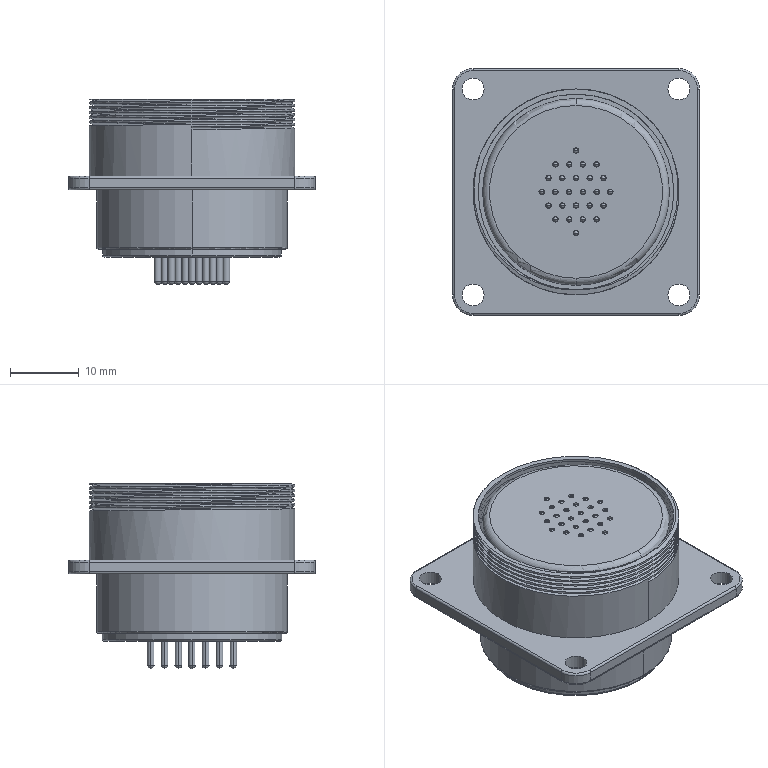Part | STEP file | WS28K26Z | 1 solid | 356 faces | box 36 x 36 x 27 mm | volume 15562 mm3 | cylinder 198 | sphere 104 | plane 38 | torus 14 | spline 2 | commonest cylinder face diameters 0.6 x60 0.8 x52 1 x52 30 x14 3.2 x8 6 x4